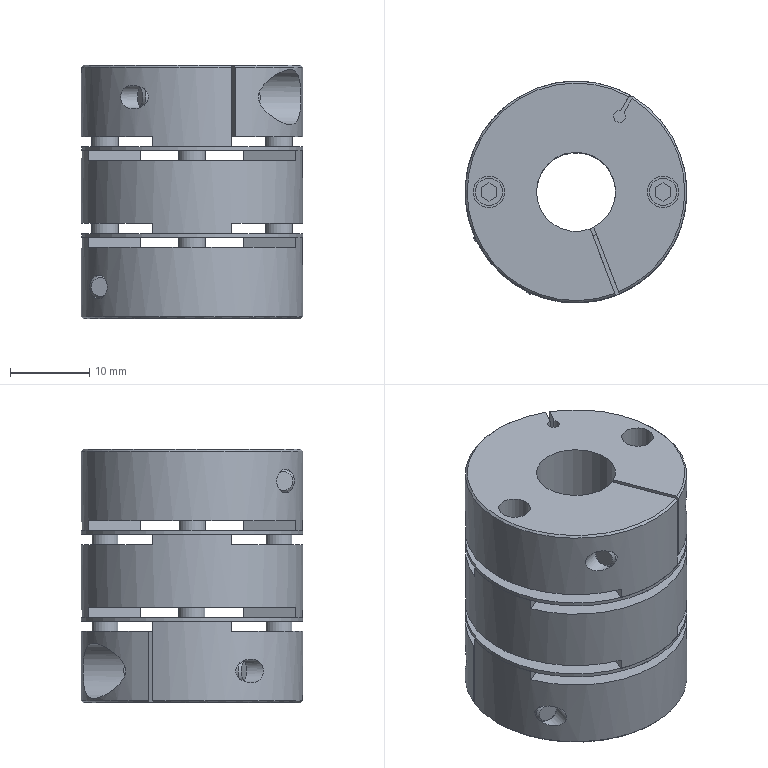Part | STEP file | 1 solid | 148 faces | box 28 x 28 x 32 mm | volume 13816 mm3 | plane 96 | cylinder 46 | cone 6 | commonest cylinder face diameters 3.429 x12 14 x8 28 x7 3 x4 4 x4 12 x3